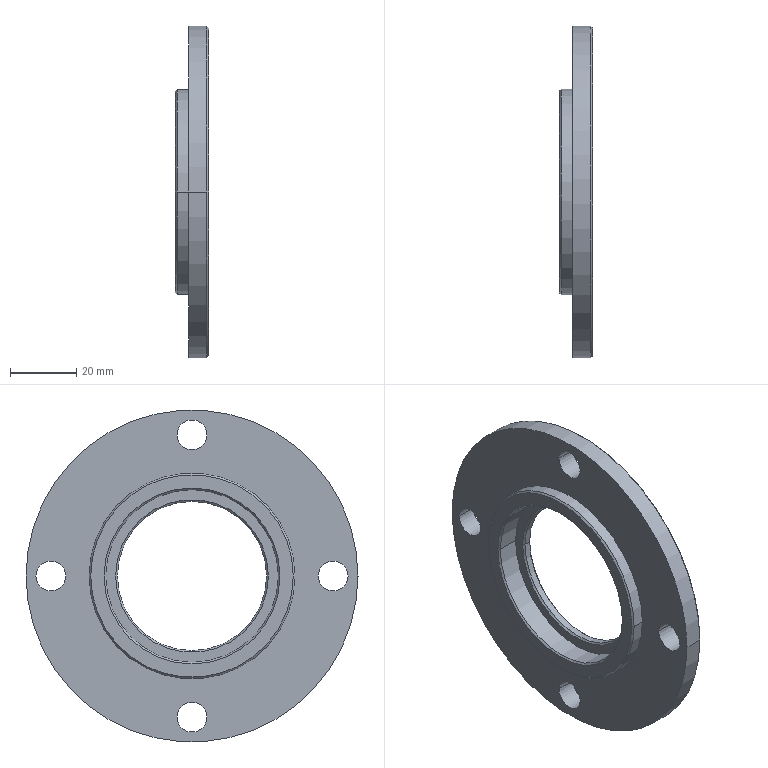Part | SolidWorks | features BaseBody 1 | 1 solid | 30 faces | box 10 x 100 x 100 mm | volume 37917 mm3 | cylinder 16 | cone 10 | plane 4 | commonest cylinder face diameters 9 x8 45 x2 52 x2 62 x2 100 x2
STEP:
#1=CARTESIAN_POINT('',(5.5,-22.5,0.));
#2=VERTEX_POINT('',#1);
#3=CARTESIAN_POINT('',(5.5,22.5,0.));
#4=VERTEX_POINT('',#3);
#5=CARTESIAN_POINT('',(5.5,0.,0.));
#6=DIRECTION('',(1.,0.,0.));
#7=DIRECTION('',(0.,-1.,0.));
#8=AXIS2_PLACEMENT_3D('',#5,#6,#7);
#9=CIRCLE('',#8,22.5);
#10=EDGE_CURVE('',#2,#4,#9,.T.);
#11=ORIENTED_EDGE('',*,*,#10,.F.);
#12=CARTESIAN_POINT('',(6.,-23.,0.));
#13=VERTEX_POINT('',#12);
#14=CARTESIAN_POINT('',(6.,-23.,0.));
#15=DIRECTION('',(0.7071,-0.7071,0.));
#16=VECTOR('',#15,1000.);
#17=LINE('',#14,#16);
#18=EDGE_CURVE('',#2,#13,#17,.T.);
#19=ORIENTED_EDGE('',*,*,#18,.T.);
#20=CARTESIAN_POINT('',(6.,23.,0.));
#21=VERTEX_POINT('',#20);
#22=CARTESIAN_POINT('',(6.,0.,0.));
#23=DIRECTION('',(-1.,0.,0.));
#24=DIRECTION('',(0.,1.,0.));
#25=AXIS2_PLACEMENT_3D('',#22,#23,#24);
#26=CIRCLE('',#25,23.);
#27=EDGE_CURVE('',#21,#13,#26,.T.);
#28=ORIENTED_EDGE('',*,*,#27,.F.);
#29=CARTESIAN_POINT('',(6.,23.,0.));
#30=DIRECTION('',(0.7071,0.7071,0.));
#31=VECTOR('',#30,1000.);
#32=LINE('',#29,#31);
#33=EDGE_CURVE('',#4,#21,#32,.T.);
#34=ORIENTED_EDGE('',*,*,#33,.F.);
#35=EDGE_LOOP('',(#11,#19,#28,#34));
#36=FACE_OUTER_BOUND('',#35,.T.);
#37=CARTESIAN_POINT('',(6.,0.,0.));
#38=DIRECTION('',(1.,0.,0.));
#39=DIRECTION('',(0.,1.,0.));
#40=AXIS2_PLACEMENT_3D('',#37,#38,#39);
#41=CONICAL_SURFACE('',#40,23.,0.7854);
#42=ADVANCED_FACE('',(#36),#41,.F.);
#43=CARTESIAN_POINT('',(6.,47.,0.));
#44=VERTEX_POINT('',#43);
#45=CARTESIAN_POINT('',(6.,38.,0.));
#46=VERTEX_POINT('',#45);
#47=CARTESIAN_POINT('',(6.,42.5,0.));
#48=DIRECTION('',(-1.,0.,0.));
#49=DIRECTION('',(0.,-1.,0.));
#50=AXIS2_PLACEMENT_3D('',#47,#48,#49);
#51=CIRCLE('',#50,4.5);
#52=EDGE_CURVE('',#44,#46,#51,.T.);
#53=ORIENTED_EDGE('',*,*,#52,.F.);
#54=CARTESIAN_POINT('',(0.,47.,0.));
#55=VERTEX_POINT('',#54);
#56=CARTESIAN_POINT('',(141.774,47.,0.));
#57=DIRECTION('',(-1.,0.,0.));
#58=VECTOR('',#57,1000.);
#59=LINE('',#56,#58);
#60=EDGE_CURVE('',#44,#55,#59,.T.);
#61=ORIENTED_EDGE('',*,*,#60,.T.);
#62=CARTESIAN_POINT('',(0.,38.,0.));
#63=VERTEX_POINT('',#62);
#64=CARTESIAN_POINT('',(0.,42.5,0.));
#65=DIRECTION('',(1.,0.,0.));
#66=DIRECTION('',(0.,-1.,0.));
#67=AXIS2_PLACEMENT_3D('',#64,#65,#66);
#68=CIRCLE('',#67,4.5);
#69=EDGE_CURVE('',#63,#55,#68,.T.);
#70=ORIENTED_EDGE('',*,*,#69,.F.);
#71=CARTESIAN_POINT('',(141.774,38.,0.));
#72=DIRECTION('',(-1.,0.,0.));
#73=VECTOR('',#72,1000.);
#74=LINE('',#71,#73);
#75=EDGE_CURVE('',#46,#63,#74,.T.);
#76=ORIENTED_EDGE('',*,*,#75,.F.);
#77=EDGE_LOOP('',(#53,#61,#70,#76));
#78=FACE_OUTER_BOUND('',#77,.T.);
#79=CARTESIAN_POINT('',(141.774,42.5,0.));
#80=DIRECTION('',(-1.,0.,0.));
#81=DIRECTION('',(0.,-1.,0.));
#82=AXIS2_PLACEMENT_3D('',#79,#80,#81);
#83=CYLINDRICAL_SURFACE('',#82,4.5);
#84=ADVANCED_FACE('',(#78),#83,.F.);
#85=CARTESIAN_POINT('',(6.,4.5,42.5));
#86=VERTEX_POINT('',#85);
#87=CARTESIAN_POINT('',(6.,-4.5,42.5));
#88=VERTEX_POINT('',#87);
#89=CARTESIAN_POINT('',(6.,0.,42.5));
#90=DIRECTION('',(-1.,0.,0.));
#91=DIRECTION('',(0.,-1.,0.));
#92=AXIS2_PLACEMENT_3D('',#89,#90,#91);
#93=CIRCLE('',#92,4.5);
#94=EDGE_CURVE('',#86,#88,#93,.T.);
#95=ORIENTED_EDGE('',*,*,#94,.F.);
#96=CARTESIAN_POINT('',(0.,4.5,42.5));
#97=VERTEX_POINT('',#96);
#98=CARTESIAN_POINT('',(141.774,4.5,42.5));
#99=DIRECTION('',(-1.,0.,0.));
#100=VECTOR('',#99,1000.);
#101=LINE('',#98,#100);
#102=EDGE_CURVE('',#86,#97,#101,.T.);
#103=ORIENTED_EDGE('',*,*,#102,.T.);
#104=CARTESIAN_POINT('',(0.,-4.5,42.5));
#105=VERTEX_POINT('',#104);
#106=CARTESIAN_POINT('',(0.,0.,42.5));
#107=DIRECTION('',(1.,0.,0.));
#108=DIRECTION('',(0.,-1.,0.));
#109=AXIS2_PLACEMENT_3D('',#106,#107,#108);
#110=CIRCLE('',#109,4.5);
#111=EDGE_CURVE('',#105,#97,#110,.T.);
#112=ORIENTED_EDGE('',*,*,#111,.F.);
#113=CARTESIAN_POINT('',(141.774,-4.5,42.5));
#114=DIRECTION('',(-1.,0.,0.));
#115=VECTOR('',#114,1000.);
#116=LINE('',#113,#115);
#117=EDGE_CURVE('',#88,#105,#116,.T.);
#118=ORIENTED_EDGE('',*,*,#117,.F.);
#119=EDGE_LOOP('',(#95,#103,#112,#118));
#120=FACE_OUTER_BOUND('',#119,.T.);
#121=CARTESIAN_POINT('',(141.774,0.,42.5));
#122=DIRECTION('',(-1.,0.,0.));
#123=DIRECTION('',(0.,-1.,0.));
#124=AXIS2_PLACEMENT_3D('',#121,#122,#123);
#125=CYLINDRICAL_SURFACE('',#124,4.5);
#126=ADVANCED_FACE('',(#120),#125,.F.);
#127=CARTESIAN_POINT('',(6.,-38.,0.));
#128=VERTEX_POINT('',#127);
#129=CARTESIAN_POINT('',(6.,-47.,0.));
#130=VERTEX_POINT('',#129);
#131=CARTESIAN_POINT('',(6.,-42.5,0.));
#132=DIRECTION('',(-1.,0.,0.));
#133=DIRECTION('',(0.,-1.,0.));
#134=AXIS2_PLACEMENT_3D('',#131,#132,#133);
#135=CIRCLE('',#134,4.5);
#136=EDGE_CURVE('',#128,#130,#135,.T.);
#137=ORIENTED_EDGE('',*,*,#136,.F.);
#138=CARTESIAN_POINT('',(0.,-38.,0.));
#139=VERTEX_POINT('',#138);
#140=CARTESIAN_POINT('',(141.774,-38.,0.));
#141=DIRECTION('',(-1.,0.,0.));
#142=VECTOR('',#141,1000.);
#143=LINE('',#140,#142);
#144=EDGE_CURVE('',#128,#139,#143,.T.);
#145=ORIENTED_EDGE('',*,*,#144,.T.);
#146=CARTESIAN_POINT('',(0.,-47.,0.));
#147=VERTEX_POINT('',#146);
#148=CARTESIAN_POINT('',(0.,-42.5,0.));
#149=DIRECTION('',(1.,0.,0.));
#150=DIRECTION('',(0.,-1.,0.));
#151=AXIS2_PLACEMENT_3D('',#148,#149,#150);
#152=CIRCLE('',#151,4.5);
#153=EDGE_CURVE('',#147,#139,#152,.T.);
#154=ORIENTED_EDGE('',*,*,#153,.F.);
#155=CARTESIAN_POINT('',(141.774,-47.,0.));
#156=DIRECTION('',(-1.,0.,0.));
#157=VECTOR('',#156,1000.);
#158=LINE('',#155,#157);
#159=EDGE_CURVE('',#130,#147,#158,.T.);
#160=ORIENTED_EDGE('',*,*,#159,.F.);
#161=EDGE_LOOP('',(#137,#145,#154,#160));
#162=FACE_OUTER_BOUND('',#161,.T.);
#163=CARTESIAN_POINT('',(141.774,-42.5,0.));
#164=DIRECTION('',(-1.,0.,0.));
#165=DIRECTION('',(0.,-1.,0.));
#166=AXIS2_PLACEMENT_3D('',#163,#164,#165);
#167=CYLINDRICAL_SURFACE('',#166,4.5);
#168=ADVANCED_FACE('',(#162),#167,.F.);
#169=CARTESIAN_POINT('',(6.,4.5,-42.5));
#170=VERTEX_POINT('',#169);
#171=CARTESIAN_POINT('',(6.,-4.5,-42.5));
#172=VERTEX_POINT('',#171);
#173=CARTESIAN_POINT('',(6.,0.,-42.5));
#174=DIRECTION('',(-1.,0.,0.));
#175=DIRECTION('',(0.,-1.,0.));
#176=AXIS2_PLACEMENT_3D('',#173,#174,#175);
#177=CIRCLE('',#176,4.5);
#178=EDGE_CURVE('',#170,#172,#177,.T.);
#179=ORIENTED_EDGE('',*,*,#178,.F.);
#180=CARTESIAN_POINT('',(0.,4.5,-42.5));
#181=VERTEX_POINT('',#180);
#182=CARTESIAN_POINT('',(141.774,4.5,-42.5));
#183=DIRECTION('',(-1.,0.,0.));
#184=VECTOR('',#183,1000.);
#185=LINE('',#182,#184);
#186=EDGE_CURVE('',#170,#181,#185,.T.);
#187=ORIENTED_EDGE('',*,*,#186,.T.);
#188=CARTESIAN_POINT('',(0.,-4.5,-42.5));
#189=VERTEX_POINT('',#188);
#190=CARTESIAN_POINT('',(0.,0.,-42.5));
#191=DIRECTION('',(1.,0.,0.));
#192=DIRECTION('',(0.,-1.,0.));
#193=AXIS2_PLACEMENT_3D('',#190,#191,#192);
#194=CIRCLE('',#193,4.5);
#195=EDGE_CURVE('',#189,#181,#194,.T.);
#196=ORIENTED_EDGE('',*,*,#195,.F.);
#197=CARTESIAN_POINT('',(141.774,-4.5,-42.5));
#198=DIRECTION('',(-1.,0.,0.));
#199=VECTOR('',#198,1000.);
#200=LINE('',#197,#199);
#201=EDGE_CURVE('',#172,#189,#200,.T.);
#202=ORIENTED_EDGE('',*,*,#201,.F.);
#203=EDGE_LOOP('',(#179,#187,#196,#202));
#204=FACE_OUTER_BOUND('',#203,.T.);
#205=CARTESIAN_POINT('',(141.774,0.,-42.5));
#206=DIRECTION('',(-1.,0.,0.));
#207=DIRECTION('',(0.,-1.,0.));
#208=AXIS2_PLACEMENT_3D('',#205,#206,#207);
#209=CYLINDRICAL_SURFACE('',#208,4.5);
#210=ADVANCED_FACE('',(#204),#209,.F.);
#211=CARTESIAN_POINT('',(6.,49.5,0.));
#212=VERTEX_POINT('',#211);
#213=CARTESIAN_POINT('',(6.,-49.5,0.));
#214=VERTEX_POINT('',#213);
#215=CARTESIAN_POINT('',(6.,0.,0.));
#216=DIRECTION('',(1.,0.,0.));
#217=DIRECTION('',(0.,-1.,0.));
#218=AXIS2_PLACEMENT_3D('',#215,#216,#217);
#219=CIRCLE('',#218,49.5);
#220=EDGE_CURVE('',#212,#214,#219,.T.);
#221=ORIENTED_EDGE('',*,*,#220,.F.);
#222=CARTESIAN_POINT('',(5.5,50.,0.));
#223=VERTEX_POINT('',#222);
#224=CARTESIAN_POINT('',(5.5,50.,0.));
#225=DIRECTION('',(-0.7071,0.7071,0.));
#226=VECTOR('',#225,1000.);
#227=LINE('',#224,#226);
#228=EDGE_CURVE('',#212,#223,#227,.T.);
#229=ORIENTED_EDGE('',*,*,#228,.T.);
#230=CARTESIAN_POINT('',(5.5,-50.,0.));
#231=VERTEX_POINT('',#230);
#232=CARTESIAN_POINT('',(5.5,0.,0.));
#233=DIRECTION('',(1.,0.,0.));
#234=DIRECTION('',(0.,-1.,0.));
#235=AXIS2_PLACEMENT_3D('',#232,#233,#234);
#236=CIRCLE('',#235,50.);
#237=EDGE_CURVE('',#223,#231,#236,.T.);
#238=ORIENTED_EDGE('',*,*,#237,.T.);
#239=CARTESIAN_POINT('',(5.5,-50.,0.));
#240=DIRECTION('',(-0.7071,-0.7071,0.));
#241=VECTOR('',#240,1000.);
#242=LINE('',#239,#241);
#243=EDGE_CURVE('',#214,#231,#242,.T.);
#244=ORIENTED_EDGE('',*,*,#243,.F.);
#245=EDGE_LOOP('',(#221,#229,#238,#244));
#246=FACE_OUTER_BOUND('',#245,.T.);
#247=CARTESIAN_POINT('',(5.5,0.,0.));
#248=DIRECTION('',(-1.,0.,0.));
#249=DIRECTION('',(0.,-1.,0.));
#250=AXIS2_PLACEMENT_3D('',#247,#248,#249);
#251=CONICAL_SURFACE('',#250,50.,0.7854);
#252=ADVANCED_FACE('',(#246),#251,.T.);
#253=CARTESIAN_POINT('',(3.5,-22.5,0.));
#254=VERTEX_POINT('',#253);
#255=CARTESIAN_POINT('',(3.5,22.5,0.));
#256=VERTEX_POINT('',#255);
#257=CARTESIAN_POINT('',(3.5,0.,0.));
#258=DIRECTION('',(1.,0.,0.));
#259=DIRECTION('',(0.,1.,0.));
#260=AXIS2_PLACEMENT_3D('',#257,#258,#259);
#261=CIRCLE('',#260,22.5);
#262=EDGE_CURVE('',#254,#256,#261,.T.);
#263=ORIENTED_EDGE('',*,*,#262,.F.);
#264=CARTESIAN_POINT('',(4.5,-22.5,0.));
#265=DIRECTION('',(1.,0.,0.));
#266=VECTOR('',#265,1000.);
#267=LINE('',#264,#266);
#268=EDGE_CURVE('',#254,#2,#267,.T.);
#269=ORIENTED_EDGE('',*,*,#268,.T.);
#270=ORIENTED_EDGE('',*,*,#10,.T.);
#271=CARTESIAN_POINT('',(4.5,22.5,0.));
#272=DIRECTION('',(1.,0.,0.));
#273=VECTOR('',#272,1000.);
#274=LINE('',#271,#273);
#275=EDGE_CURVE('',#256,#4,#274,.T.);
#276=ORIENTED_EDGE('',*,*,#275,.F.);
#277=EDGE_LOOP('',(#263,#269,#270,#276));
#278=FACE_OUTER_BOUND('',#277,.T.);
#279=CARTESIAN_POINT('',(4.5,0.,0.));
#280=DIRECTION('',(1.,0.,0.));
#281=DIRECTION('',(0.,1.,0.));
#282=AXIS2_PLACEMENT_3D('',#279,#280,#281);
#283=CYLINDRICAL_SURFACE('',#282,22.5);
#284=ADVANCED_FACE('',(#278),#283,.F.);
#285=CARTESIAN_POINT('',(0.,-50.,0.));
#286=VERTEX_POINT('',#285);
#287=CARTESIAN_POINT('',(0.,50.,0.));
#288=VERTEX_POINT('',#287);
#289=CARTESIAN_POINT('',(0.,0.,0.));
#290=DIRECTION('',(-1.,0.,0.));
#291=DIRECTION('',(0.,1.,0.));
#292=AXIS2_PLACEMENT_3D('',#289,#290,#291);
#293=CIRCLE('',#292,50.);
#294=EDGE_CURVE('',#286,#288,#293,.T.);
#295=ORIENTED_EDGE('',*,*,#294,.F.);
#296=CARTESIAN_POINT('',(3.,-50.,0.));
#297=DIRECTION('',(1.,0.,0.));
#298=VECTOR('',#297,1000.);
#299=LINE('',#296,#298);
#300=EDGE_CURVE('',#286,#231,#299,.T.);
#301=ORIENTED_EDGE('',*,*,#300,.T.);
#302=ORIENTED_EDGE('',*,*,#237,.F.);
#303=CARTESIAN_POINT('',(3.,50.,0.));
#304=DIRECTION('',(1.,0.,0.));
#305=VECTOR('',#304,1000.);
#306=LINE('',#303,#305);
#307=EDGE_CURVE('',#288,#223,#306,.T.);
#308=ORIENTED_EDGE('',*,*,#307,.F.);
#309=EDGE_LOOP('',(#295,#301,#302,#308));
#310=FACE_OUTER_BOUND('',#309,.T.);
#311=CARTESIAN_POINT('',(3.,0.,0.));
#312=DIRECTION('',(1.,0.,0.));
#313=DIRECTION('',(0.,1.,0.));
#314=AXIS2_PLACEMENT_3D('',#311,#312,#313);
#315=CYLINDRICAL_SURFACE('',#314,50.);
#316=ADVANCED_FACE('',(#310),#315,.T.);
#317=ORIENTED_EDGE('',*,*,#262,.T.);
#318=CARTESIAN_POINT('',(3.,23.,0.));
#319=VERTEX_POINT('',#318);
#320=CARTESIAN_POINT('',(3.,23.,0.));
#321=DIRECTION('',(-0.7071,0.7071,0.));
#322=VECTOR('',#321,1000.);
#323=LINE('',#320,#322);
#324=EDGE_CURVE('',#256,#319,#323,.T.);
#325=ORIENTED_EDGE('',*,*,#324,.T.);
#326=CARTESIAN_POINT('',(3.,-23.,0.));
#327=VERTEX_POINT('',#326);
#328=CARTESIAN_POINT('',(3.,0.,0.));
#329=DIRECTION('',(1.,0.,0.));
#330=DIRECTION('',(0.,-1.,0.));
#331=AXIS2_PLACEMENT_3D('',#328,#329,#330);
#332=CIRCLE('',#331,23.);
#333=EDGE_CURVE('',#327,#319,#332,.T.);
#334=ORIENTED_EDGE('',*,*,#333,.F.);
#335=CARTESIAN_POINT('',(3.,-23.,0.));
#336=DIRECTION('',(-0.7071,-0.7071,0.));
#337=VECTOR('',#336,1000.);
#338=LINE('',#335,#337);
#339=EDGE_CURVE('',#254,#327,#338,.T.);
#340=ORIENTED_EDGE('',*,*,#339,.F.);
#341=EDGE_LOOP('',(#317,#325,#334,#340));
#342=FACE_OUTER_BOUND('',#341,.T.);
#343=CARTESIAN_POINT('',(3.,0.,0.));
#344=DIRECTION('',(-1.,0.,0.));
#345=DIRECTION('',(0.,-1.,0.));
#346=AXIS2_PLACEMENT_3D('',#343,#344,#345);
#347=CONICAL_SURFACE('',#346,23.,0.7854);
#348=ADVANCED_FACE('',(#342),#347,.F.);
#349=CARTESIAN_POINT('',(-3.5,31.,0.));
#350=VERTEX_POINT('',#349);
#351=CARTESIAN_POINT('',(-3.5,-31.,0.));
#352=VERTEX_POINT('',#351);
#353=CARTESIAN_POINT('',(-3.5,0.,0.));
#354=DIRECTION('',(1.,0.,0.));
#355=DIRECTION('',(0.,1.,0.));
#356=AXIS2_PLACEMENT_3D('',#353,#354,#355);
#357=CIRCLE('',#356,31.);
#358=EDGE_CURVE('',#350,#352,#357,.T.);
#359=ORIENTED_EDGE('',*,*,#358,.T.);
#360=CARTESIAN_POINT('',(0.,-31.,0.));
#361=VERTEX_POINT('',#360);
#362=CARTESIAN_POINT('',(-2.,-31.,0.));
#363=DIRECTION('',(1.,0.,0.));
#364=VECTOR('',#363,1000.);
#365=LINE('',#362,#364);
#366=EDGE_CURVE('',#352,#361,#365,.T.);
#367=ORIENTED_EDGE('',*,*,#366,.T.);
#368=CARTESIAN_POINT('',(0.,31.,0.));
#369=VERTEX_POINT('',#368);
#370=CARTESIAN_POINT('',(0.,0.,0.));
#371=DIRECTION('',(1.,0.,0.));
#372=DIRECTION('',(0.,1.,0.));
#373=AXIS2_PLACEMENT_3D('',#370,#371,#372);
#374=CIRCLE('',#373,31.);
#375=EDGE_CURVE('',#369,#361,#374,.T.);
#376=ORIENTED_EDGE('',*,*,#375,.F.);
#377=CARTESIAN_POINT('',(-2.,31.,0.));
#378=DIRECTION('',(1.,0.,0.));
#379=VECTOR('',#378,1000.);
#380=LINE('',#377,#379);
#381=EDGE_CURVE('',#350,#369,#380,.T.);
#382=ORIENTED_EDGE('',*,*,#381,.F.);
#383=EDGE_LOOP('',(#359,#367,#376,#382));
#384=FACE_OUTER_BOUND('',#383,.T.);
#385=CARTESIAN_POINT('',(-2.,0.,0.));
#386=DIRECTION('',(1.,0.,0.));
#387=DIRECTION('',(0.,1.,0.));
#388=AXIS2_PLACEMENT_3D('',#385,#386,#387);
#389=CYLINDRICAL_SURFACE('',#388,31.);
#390=ADVANCED_FACE('',(#384),#389,.T.);
#391=CARTESIAN_POINT('',(-4.,30.5,0.));
#392=VERTEX_POINT('',#391);
#393=CARTESIAN_POINT('',(-4.,-30.5,0.));
#394=VERTEX_POINT('',#393);
#395=CARTESIAN_POINT('',(-4.,0.,0.));
#396=DIRECTION('',(1.,0.,0.));
#397=DIRECTION('',(0.,1.,0.));
#398=AXIS2_PLACEMENT_3D('',#395,#396,#397);
#399=CIRCLE('',#398,30.5);
#400=EDGE_CURVE('',#392,#394,#399,.T.);
#401=ORIENTED_EDGE('',*,*,#400,.T.);
#402=CARTESIAN_POINT('',(-3.5,-31.,0.));
#403=DIRECTION('',(0.7071,-0.7071,0.));
#404=VECTOR('',#403,1000.);
#405=LINE('',#402,#404);
#406=EDGE_CURVE('',#394,#352,#405,.T.);
#407=ORIENTED_EDGE('',*,*,#406,.T.);
#408=ORIENTED_EDGE('',*,*,#358,.F.);
#409=CARTESIAN_POINT('',(-3.5,31.,0.));
#410=DIRECTION('',(0.7071,0.7071,0.));
#411=VECTOR('',#410,1000.);
#412=LINE('',#409,#411);
#413=EDGE_CURVE('',#392,#350,#412,.T.);
#414=ORIENTED_EDGE('',*,*,#413,.F.);
#415=EDGE_LOOP('',(#401,#407,#408,#414));
#416=FACE_OUTER_BOUND('',#415,.T.);
#417=CARTESIAN_POINT('',(-3.5,0.,0.));
#418=DIRECTION('',(1.,0.,0.));
#419=DIRECTION('',(0.,1.,0.));
#420=AXIS2_PLACEMENT_3D('',#417,#418,#419);
#421=CONICAL_SURFACE('',#420,31.,0.7854);
#422=ADVANCED_FACE('',(#416),#421,.T.);
#423=CARTESIAN_POINT('',(-3.5,-26.,0.));
#424=VERTEX_POINT('',#423);
#425=CARTESIAN_POINT('',(-3.5,26.,0.));
#426=VERTEX_POINT('',#425);
#427=CARTESIAN_POINT('',(-3.5,0.,0.));
#428=DIRECTION('',(1.,0.,0.));
#429=DIRECTION('',(0.,1.,0.));
#430=AXIS2_PLACEMENT_3D('',#427,#428,#429);
#431=CIRCLE('',#430,26.);
#432=EDGE_CURVE('',#424,#426,#431,.T.);
#433=ORIENTED_EDGE('',*,*,#432,.F.);
#434=CARTESIAN_POINT('',(3.,-26.,0.));
#435=VERTEX_POINT('',#434);
#436=CARTESIAN_POINT('',(-0.5,-26.,0.));
#437=DIRECTION('',(1.,0.,0.));
#438=VECTOR('',#437,1000.);
#439=LINE('',#436,#438);
#440=EDGE_CURVE('',#424,#435,#439,.T.);
#441=ORIENTED_EDGE('',*,*,#440,.T.);
#442=CARTESIAN_POINT('',(3.,26.,0.));
#443=VERTEX_POINT('',#442);
#444=CARTESIAN_POINT('',(3.,0.,0.));
#445=DIRECTION('',(-1.,0.,0.));
#446=DIRECTION('',(0.,1.,0.));
#447=AXIS2_PLACEMENT_3D('',#444,#445,#446);
#448=CIRCLE('',#447,26.);
#449=EDGE_CURVE('',#443,#435,#448,.T.);
#450=ORIENTED_EDGE('',*,*,#449,.F.);
#451=CARTESIAN_POINT('',(-0.5,26.,0.));
#452=DIRECTION('',(1.,0.,0.));
#453=VECTOR('',#452,1000.);
#454=LINE('',#451,#453);
#455=EDGE_CURVE('',#426,#443,#454,.T.);
#456=ORIENTED_EDGE('',*,*,#455,.F.);
#457=EDGE_LOOP('',(#433,#441,#450,#456));
#458=FACE_OUTER_BOUND('',#457,.T.);
#459=CARTESIAN_POINT('',(-0.5,0.,0.));
#460=DIRECTION('',(1.,0.,0.));
#461=DIRECTION('',(0.,1.,0.));
#462=AXIS2_PLACEMENT_3D('',#459,#460,#461);
#463=CYLINDRICAL_SURFACE('',#462,26.);
#464=ADVANCED_FACE('',(#458),#463,.F.);
#465=ORIENTED_EDGE('',*,*,#432,.T.);
#466=CARTESIAN_POINT('',(-4.,26.5,0.));
#467=VERTEX_POINT('',#466);
#468=CARTESIAN_POINT('',(-4.,26.5,0.));
#469=DIRECTION('',(-0.7071,0.7071,0.));
#470=VECTOR('',#469,1000.);
#471=LINE('',#468,#470);
#472=EDGE_CURVE('',#426,#467,#471,.T.);
#473=ORIENTED_EDGE('',*,*,#472,.T.);
#474=CARTESIAN_POINT('',(-4.,-26.5,0.));
#475=VERTEX_POINT('',#474);
#476=CARTESIAN_POINT('',(-4.,0.,0.));
#477=DIRECTION('',(1.,0.,0.));
#478=DIRECTION('',(0.,-1.,0.));
#479=AXIS2_PLACEMENT_3D('',#476,#477,#478);
#480=CIRCLE('',#479,26.5);
#481=EDGE_CURVE('',#475,#467,#480,.T.);
#482=ORIENTED_EDGE('',*,*,#481,.F.);
#483=CARTESIAN_POINT('',(-4.,-26.5,0.));
#484=DIRECTION('',(-0.7071,-0.7071,0.));
#485=VECTOR('',#484,1000.);
#486=LINE('',#483,#485);
#487=EDGE_CURVE('',#424,#475,#486,.T.);
#488=ORIENTED_EDGE('',*,*,#487,.F.);
#489=EDGE_LOOP('',(#465,#473,#482,#488));
#490=FACE_OUTER_BOUND('',#489,.T.);
#491=CARTESIAN_POINT('',(-4.,0.,0.));
#492=DIRECTION('',(-1.,0.,0.));
#493=DIRECTION('',(0.,-1.,0.));
#494=AXIS2_PLACEMENT_3D('',#491,#492,#493);
#495=CONICAL_SURFACE('',#494,26.5,0.7854);
#496=ADVANCED_FACE('',(#490),#495,.F.);
#497=ORIENTED_EDGE('',*,*,#27,.T.);
#498=CARTESIAN_POINT('',(6.,0.,0.));
#499=DIRECTION('',(-1.,0.,0.));
#500=DIRECTION('',(0.,1.,0.));
#501=AXIS2_PLACEMENT_3D('',#498,#499,#500);
#502=CIRCLE('',#501,23.);
#503=EDGE_CURVE('',#13,#21,#502,.T.);
#504=ORIENTED_EDGE('',*,*,#503,.T.);
#505=EDGE_LOOP('',(#497,#504));
#506=FACE_BOUND('',#505,.T.);
#507=CARTESIAN_POINT('',(6.,42.5,0.));
#508=DIRECTION('',(-1.,0.,0.));
#509=DIRECTION('',(0.,-1.,0.));
#510=AXIS2_PLACEMENT_3D('',#507,#508,#509);
#511=CIRCLE('',#510,4.5);
#512=EDGE_CURVE('',#46,#44,#511,.T.);
#513=ORIENTED_EDGE('',*,*,#512,.T.);
#514=ORIENTED_EDGE('',*,*,#52,.T.);
#515=EDGE_LOOP('',(#513,#514));
#516=FACE_BOUND('',#515,.T.);
#517=CARTESIAN_POINT('',(6.,0.,42.5));
#518=DIRECTION('',(-1.,0.,0.));
#519=DIRECTION('',(0.,-1.,0.));
#520=AXIS2_PLACEMENT_3D('',#517,#518,#519);
#521=CIRCLE('',#520,4.5);
#522=EDGE_CURVE('',#88,#86,#521,.T.);
#523=ORIENTED_EDGE('',*,*,#522,.T.);
#524=ORIENTED_EDGE('',*,*,#94,.T.);
#525=EDGE_LOOP('',(#523,#524));
#526=FACE_BOUND('',#525,.T.);
#527=CARTESIAN_POINT('',(6.,-42.5,0.));
#528=DIRECTION('',(-1.,0.,0.));
#529=DIRECTION('',(0.,-1.,0.));
#530=AXIS2_PLACEMENT_3D('',#527,#528,#529);
#531=CIRCLE('',#530,4.5);
#532=EDGE_CURVE('',#130,#128,#531,.T.);
#533=ORIENTED_EDGE('',*,*,#532,.T.);
#534=ORIENTED_EDGE('',*,*,#136,.T.);
#535=EDGE_LOOP('',(#533,#534));
#536=FACE_BOUND('',#535,.T.);
#537=CARTESIAN_POINT('',(6.,0.,-42.5));
#538=DIRECTION('',(-1.,0.,0.));
#539=DIRECTION('',(0.,-1.,0.));
#540=AXIS2_PLACEMENT_3D('',#537,#538,#539);
#541=CIRCLE('',#540,4.5);
#542=EDGE_CURVE('',#172,#170,#541,.T.);
#543=ORIENTED_EDGE('',*,*,#542,.T.);
#544=ORIENTED_EDGE('',*,*,#178,.T.);
#545=EDGE_LOOP('',(#543,#544));
#546=FACE_BOUND('',#545,.T.);
#547=CARTESIAN_POINT('',(6.,0.,0.));
#548=DIRECTION('',(1.,0.,0.));
#549=DIRECTION('',(0.,-1.,0.));
#550=AXIS2_PLACEMENT_3D('',#547,#548,#549);
#551=CIRCLE('',#550,49.5);
#552=EDGE_CURVE('',#214,#212,#551,.T.);
#553=ORIENTED_EDGE('',*,*,#552,.T.);
#554=ORIENTED_EDGE('',*,*,#220,.T.);
#555=EDGE_LOOP('',(#553,#554));
#556=FACE_OUTER_BOUND('',#555,.T.);
#557=CARTESIAN_POINT('',(6.,22.5,0.));
#558=DIRECTION('',(1.,0.,0.));
#559=DIRECTION('',(0.,1.,0.));
#560=AXIS2_PLACEMENT_3D('',#557,#558,#559);
#561=PLANE('',#560);
#562=ADVANCED_FACE('',(#506,#516,#526,#536,#546,#556),#561,.T.);
#563=ORIENTED_EDGE('',*,*,#18,.F.);
#564=CARTESIAN_POINT('',(5.5,0.,0.));
#565=DIRECTION('',(1.,0.,0.));
#566=DIRECTION('',(0.,-1.,0.));
#567=AXIS2_PLACEMENT_3D('',#564,#565,#566);
#568=CIRCLE('',#567,22.5);
#569=EDGE_CURVE('',#4,#2,#568,.T.);
#570=ORIENTED_EDGE('',*,*,#569,.F.);
#571=ORIENTED_EDGE('',*,*,#33,.T.);
#572=ORIENTED_EDGE('',*,*,#503,.F.);
#573=EDGE_LOOP('',(#563,#570,#571,#572));
#574=FACE_OUTER_BOUND('',#573,.T.);
#575=CARTESIAN_POINT('',(6.,0.,0.));
#576=DIRECTION('',(1.,0.,0.));
#577=DIRECTION('',(0.,1.,0.));
#578=AXIS2_PLACEMENT_3D('',#575,#576,#577);
#579=CONICAL_SURFACE('',#578,23.,0.7854);
#580=ADVANCED_FACE('',(#574),#579,.F.);
#581=ORIENTED_EDGE('',*,*,#60,.F.);
#582=ORIENTED_EDGE('',*,*,#512,.F.);
#583=ORIENTED_EDGE('',*,*,#75,.T.);
#584=CARTESIAN_POINT('',(0.,42.5,0.));
#585=DIRECTION('',(1.,0.,0.));
#586=DIRECTION('',(0.,-1.,0.));
#587=AXIS2_PLACEMENT_3D('',#584,#585,#586);
#588=CIRCLE('',#587,4.5);
#589=EDGE_CURVE('',#55,#63,#588,.T.);
#590=ORIENTED_EDGE('',*,*,#589,.F.);
#591=EDGE_LOOP('',(#581,#582,#583,#590));
#592=FACE_OUTER_BOUND('',#591,.T.);
#593=CARTESIAN_POINT('',(141.774,42.5,0.));
#594=DIRECTION('',(-1.,0.,0.));
#595=DIRECTION('',(0.,-1.,0.));
#596=AXIS2_PLACEMENT_3D('',#593,#594,#595);
#597=CYLINDRICAL_SURFACE('',#596,4.5);
#598=ADVANCED_FACE('',(#592),#597,.F.);
#599=ORIENTED_EDGE('',*,*,#102,.F.);
#600=ORIENTED_EDGE('',*,*,#522,.F.);
#601=ORIENTED_EDGE('',*,*,#117,.T.);
#602=CARTESIAN_POINT('',(0.,0.,42.5));
#603=DIRECTION('',(1.,0.,0.));
#604=DIRECTION('',(0.,-1.,0.));
#605=AXIS2_PLACEMENT_3D('',#602,#603,#604);
#606=CIRCLE('',#605,4.5);
#607=EDGE_CURVE('',#97,#105,#606,.T.);
#608=ORIENTED_EDGE('',*,*,#607,.F.);
#609=EDGE_LOOP('',(#599,#600,#601,#608));
#610=FACE_OUTER_BOUND('',#609,.T.);
#611=CARTESIAN_POINT('',(141.774,0.,42.5));
#612=DIRECTION('',(-1.,0.,0.));
#613=DIRECTION('',(0.,-1.,0.));
#614=AXIS2_PLACEMENT_3D('',#611,#612,#613);
#615=CYLINDRICAL_SURFACE('',#614,4.5);
#616=ADVANCED_FACE('',(#610),#615,.F.);
#617=ORIENTED_EDGE('',*,*,#144,.F.);
#618=ORIENTED_EDGE('',*,*,#532,.F.);
#619=ORIENTED_EDGE('',*,*,#159,.T.);
#620=CARTESIAN_POINT('',(0.,-42.5,0.));
#621=DIRECTION('',(1.,0.,0.));
#622=DIRECTION('',(0.,-1.,0.));
#623=AXIS2_PLACEMENT_3D('',#620,#621,#622);
#624=CIRCLE('',#623,4.5);
#625=EDGE_CURVE('',#139,#147,#624,.T.);
#626=ORIENTED_EDGE('',*,*,#625,.F.);
#627=EDGE_LOOP('',(#617,#618,#619,#626));
#628=FACE_OUTER_BOUND('',#627,.T.);
#629=CARTESIAN_POINT('',(141.774,-42.5,0.));
#630=DIRECTION('',(-1.,0.,0.));
#631=DIRECTION('',(0.,-1.,0.));
#632=AXIS2_PLACEMENT_3D('',#629,#630,#631);
#633=CYLINDRICAL_SURFACE('',#632,4.5);
#634=ADVANCED_FACE('',(#628),#633,.F.);
#635=ORIENTED_EDGE('',*,*,#186,.F.);
#636=ORIENTED_EDGE('',*,*,#542,.F.);
#637=ORIENTED_EDGE('',*,*,#201,.T.);
#638=CARTESIAN_POINT('',(0.,0.,-42.5));
#639=DIRECTION('',(1.,0.,0.));
#640=DIRECTION('',(0.,-1.,0.));
#641=AXIS2_PLACEMENT_3D('',#638,#639,#640);
#642=CIRCLE('',#641,4.5);
#643=EDGE_CURVE('',#181,#189,#642,.T.);
#644=ORIENTED_EDGE('',*,*,#643,.F.);
#645=EDGE_LOOP('',(#635,#636,#637,#644));
#646=FACE_OUTER_BOUND('',#645,.T.);
#647=CARTESIAN_POINT('',(141.774,0.,-42.5));
#648=DIRECTION('',(-1.,0.,0.));
#649=DIRECTION('',(0.,-1.,0.));
#650=AXIS2_PLACEMENT_3D('',#647,#648,#649);
#651=CYLINDRICAL_SURFACE('',#650,4.5);
#652=ADVANCED_FACE('',(#646),#651,.F.);
#653=ORIENTED_EDGE('',*,*,#228,.F.);
#654=ORIENTED_EDGE('',*,*,#552,.F.);
#655=ORIENTED_EDGE('',*,*,#243,.T.);
#656=CARTESIAN_POINT('',(5.5,0.,0.));
#657=DIRECTION('',(1.,0.,0.));
#658=DIRECTION('',(0.,-1.,0.));
#659=AXIS2_PLACEMENT_3D('',#656,#657,#658);
#660=CIRCLE('',#659,50.);
#661=EDGE_CURVE('',#231,#223,#660,.T.);
#662=ORIENTED_EDGE('',*,*,#661,.T.);
#663=EDGE_LOOP('',(#653,#654,#655,#662));
#664=FACE_OUTER_BOUND('',#663,.T.);
#665=CARTESIAN_POINT('',(5.5,0.,0.));
#666=DIRECTION('',(-1.,0.,0.));
#667=DIRECTION('',(0.,-1.,0.));
#668=AXIS2_PLACEMENT_3D('',#665,#666,#667);
#669=CONICAL_SURFACE('',#668,50.,0.7854);
#670=ADVANCED_FACE('',(#664),#669,.T.);
#671=ORIENTED_EDGE('',*,*,#268,.F.);
#672=CARTESIAN_POINT('',(3.5,0.,0.));
#673=DIRECTION('',(1.,0.,0.));
#674=DIRECTION('',(0.,1.,0.));
#675=AXIS2_PLACEMENT_3D('',#672,#673,#674);
#676=CIRCLE('',#675,22.5);
#677=EDGE_CURVE('',#256,#254,#676,.T.);
#678=ORIENTED_EDGE('',*,*,#677,.F.);
#679=ORIENTED_EDGE('',*,*,#275,.T.);
#680=ORIENTED_EDGE('',*,*,#569,.T.);
#681=EDGE_LOOP('',(#671,#678,#679,#680));
#682=FACE_OUTER_BOUND('',#681,.T.);
#683=CARTESIAN_POINT('',(4.5,0.,0.));
#684=DIRECTION('',(1.,0.,0.));
#685=DIRECTION('',(0.,1.,0.));
#686=AXIS2_PLACEMENT_3D('',#683,#684,#685);
#687=CYLINDRICAL_SURFACE('',#686,22.5);
#688=ADVANCED_FACE('',(#682),#687,.F.);
#689=ORIENTED_EDGE('',*,*,#375,.T.);
#690=CARTESIAN_POINT('',(0.,0.,0.));
#691=DIRECTION('',(1.,0.,0.));
#692=DIRECTION('',(0.,1.,0.));
#693=AXIS2_PLACEMENT_3D('',#690,#691,#692);
#694=CIRCLE('',#693,31.);
#695=EDGE_CURVE('',#361,#369,#694,.T.);
#696=ORIENTED_EDGE('',*,*,#695,.T.);
#697=EDGE_LOOP('',(#689,#696));
#698=FACE_BOUND('',#697,.T.);
#699=ORIENTED_EDGE('',*,*,#69,.T.);
#700=ORIENTED_EDGE('',*,*,#589,.T.);
#701=EDGE_LOOP('',(#699,#700));
#702=FACE_BOUND('',#701,.T.);
#703=ORIENTED_EDGE('',*,*,#111,.T.);
#704=ORIENTED_EDGE('',*,*,#607,.T.);
#705=EDGE_LOOP('',(#703,#704));
#706=FACE_BOUND('',#705,.T.);
#707=ORIENTED_EDGE('',*,*,#153,.T.);
#708=ORIENTED_EDGE('',*,*,#625,.T.);
#709=EDGE_LOOP('',(#707,#708));
#710=FACE_BOUND('',#709,.T.);
#711=ORIENTED_EDGE('',*,*,#195,.T.);
#712=ORIENTED_EDGE('',*,*,#643,.T.);
#713=EDGE_LOOP('',(#711,#712));
#714=FACE_BOUND('',#713,.T.);
#715=CARTESIAN_POINT('',(0.,0.,0.));
#716=DIRECTION('',(-1.,0.,0.));
#717=DIRECTION('',(0.,1.,0.));
#718=AXIS2_PLACEMENT_3D('',#715,#716,#717);
#719=CIRCLE('',#718,50.);
#720=EDGE_CURVE('',#288,#286,#719,.T.);
#721=ORIENTED_EDGE('',*,*,#720,.T.);
#722=ORIENTED_EDGE('',*,*,#294,.T.);
#723=EDGE_LOOP('',(#721,#722));
#724=FACE_OUTER_BOUND('',#723,.T.);
#725=CARTESIAN_POINT('',(0.,50.,0.));
#726=DIRECTION('',(-1.,0.,0.));
#727=DIRECTION('',(0.,-1.,0.));
#728=AXIS2_PLACEMENT_3D('',#725,#726,#727);
#729=PLANE('',#728);
#730=ADVANCED_FACE('',(#698,#702,#706,#710,#714,#724),#729,.T.);
#731=ORIENTED_EDGE('',*,*,#300,.F.);
#732=ORIENTED_EDGE('',*,*,#720,.F.);
#733=ORIENTED_EDGE('',*,*,#307,.T.);
#734=ORIENTED_EDGE('',*,*,#661,.F.);
#735=EDGE_LOOP('',(#731,#732,#733,#734));
#736=FACE_OUTER_BOUND('',#735,.T.);
#737=CARTESIAN_POINT('',(3.,0.,0.));
#738=DIRECTION('',(1.,0.,0.));
#739=DIRECTION('',(0.,1.,0.));
#740=AXIS2_PLACEMENT_3D('',#737,#738,#739);
#741=CYLINDRICAL_SURFACE('',#740,50.);
#742=ADVANCED_FACE('',(#736),#741,.T.);
#743=ORIENTED_EDGE('',*,*,#324,.F.);
#744=ORIENTED_EDGE('',*,*,#677,.T.);
#745=ORIENTED_EDGE('',*,*,#339,.T.);
#746=CARTESIAN_POINT('',(3.,0.,0.));
#747=DIRECTION('',(1.,0.,0.));
#748=DIRECTION('',(0.,-1.,0.));
#749=AXIS2_PLACEMENT_3D('',#746,#747,#748);
#750=CIRCLE('',#749,23.);
#751=EDGE_CURVE('',#319,#327,#750,.T.);
#752=ORIENTED_EDGE('',*,*,#751,.F.);
#753=EDGE_LOOP('',(#743,#744,#745,#752));
#754=FACE_OUTER_BOUND('',#753,.T.);
#755=CARTESIAN_POINT('',(3.,0.,0.));
#756=DIRECTION('',(-1.,0.,0.));
#757=DIRECTION('',(0.,-1.,0.));
#758=AXIS2_PLACEMENT_3D('',#755,#756,#757);
#759=CONICAL_SURFACE('',#758,23.,0.7854);
#760=ADVANCED_FACE('',(#754),#759,.F.);
#761=ORIENTED_EDGE('',*,*,#366,.F.);
#762=CARTESIAN_POINT('',(-3.5,0.,0.));
#763=DIRECTION('',(1.,0.,0.));
#764=DIRECTION('',(0.,1.,0.));
#765=AXIS2_PLACEMENT_3D('',#762,#763,#764);
#766=CIRCLE('',#765,31.);
#767=EDGE_CURVE('',#352,#350,#766,.T.);
#768=ORIENTED_EDGE('',*,*,#767,.T.);
#769=ORIENTED_EDGE('',*,*,#381,.T.);
#770=ORIENTED_EDGE('',*,*,#695,.F.);
#771=EDGE_LOOP('',(#761,#768,#769,#770));
#772=FACE_OUTER_BOUND('',#771,.T.);
#773=CARTESIAN_POINT('',(-2.,0.,0.));
#774=DIRECTION('',(1.,0.,0.));
#775=DIRECTION('',(0.,1.,0.));
#776=AXIS2_PLACEMENT_3D('',#773,#774,#775);
#777=CYLINDRICAL_SURFACE('',#776,31.);
#778=ADVANCED_FACE('',(#772),#777,.T.);
#779=ORIENTED_EDGE('',*,*,#333,.T.);
#780=ORIENTED_EDGE('',*,*,#751,.T.);
#781=EDGE_LOOP('',(#779,#780));
#782=FACE_BOUND('',#781,.T.);
#783=ORIENTED_EDGE('',*,*,#449,.T.);
#784=CARTESIAN_POINT('',(3.,0.,0.));
#785=DIRECTION('',(-1.,0.,0.));
#786=DIRECTION('',(0.,1.,0.));
#787=AXIS2_PLACEMENT_3D('',#784,#785,#786);
#788=CIRCLE('',#787,26.);
#789=EDGE_CURVE('',#435,#443,#788,.T.);
#790=ORIENTED_EDGE('',*,*,#789,.T.);
#791=EDGE_LOOP('',(#783,#790));
#792=FACE_OUTER_BOUND('',#791,.T.);
#793=CARTESIAN_POINT('',(3.,26.,0.));
#794=DIRECTION('',(-1.,0.,0.));
#795=DIRECTION('',(0.,-1.,0.));
#796=AXIS2_PLACEMENT_3D('',#793,#794,#795);
#797=PLANE('',#796);
#798=ADVANCED_FACE('',(#782,#792),#797,.T.);
#799=ORIENTED_EDGE('',*,*,#406,.F.);
#800=CARTESIAN_POINT('',(-4.,0.,0.));
#801=DIRECTION('',(1.,0.,0.));
#802=DIRECTION('',(0.,1.,0.));
#803=AXIS2_PLACEMENT_3D('',#800,#801,#802);
#804=CIRCLE('',#803,30.5);
#805=EDGE_CURVE('',#394,#392,#804,.T.);
#806=ORIENTED_EDGE('',*,*,#805,.T.);
#807=ORIENTED_EDGE('',*,*,#413,.T.);
#808=ORIENTED_EDGE('',*,*,#767,.F.);
#809=EDGE_LOOP('',(#799,#806,#807,#808));
#810=FACE_OUTER_BOUND('',#809,.T.);
#811=CARTESIAN_POINT('',(-3.5,0.,0.));
#812=DIRECTION('',(1.,0.,0.));
#813=DIRECTION('',(0.,1.,0.));
#814=AXIS2_PLACEMENT_3D('',#811,#812,#813);
#815=CONICAL_SURFACE('',#814,31.,0.7854);
#816=ADVANCED_FACE('',(#810),#815,.T.);
#817=ORIENTED_EDGE('',*,*,#440,.F.);
#818=CARTESIAN_POINT('',(-3.5,0.,0.));
#819=DIRECTION('',(1.,0.,0.));
#820=DIRECTION('',(0.,1.,0.));
#821=AXIS2_PLACEMENT_3D('',#818,#819,#820);
#822=CIRCLE('',#821,26.);
#823=EDGE_CURVE('',#426,#424,#822,.T.);
#824=ORIENTED_EDGE('',*,*,#823,.F.);
#825=ORIENTED_EDGE('',*,*,#455,.T.);
#826=ORIENTED_EDGE('',*,*,#789,.F.);
#827=EDGE_LOOP('',(#817,#824,#825,#826));
#828=FACE_OUTER_BOUND('',#827,.T.);
#829=CARTESIAN_POINT('',(-0.5,0.,0.));
#830=DIRECTION('',(1.,0.,0.));
#831=DIRECTION('',(0.,1.,0.));
#832=AXIS2_PLACEMENT_3D('',#829,#830,#831);
#833=CYLINDRICAL_SURFACE('',#832,26.);
#834=ADVANCED_FACE('',(#828),#833,.F.);
#835=ORIENTED_EDGE('',*,*,#481,.T.);
#836=CARTESIAN_POINT('',(-4.,0.,0.));
#837=DIRECTION('',(1.,0.,0.));
#838=DIRECTION('',(0.,-1.,0.));
#839=AXIS2_PLACEMENT_3D('',#836,#837,#838);
#840=CIRCLE('',#839,26.5);
#841=EDGE_CURVE('',#467,#475,#840,.T.);
#842=ORIENTED_EDGE('',*,*,#841,.T.);
#843=EDGE_LOOP('',(#835,#842));
#844=FACE_BOUND('',#843,.T.);
#845=ORIENTED_EDGE('',*,*,#400,.F.);
#846=ORIENTED_EDGE('',*,*,#805,.F.);
#847=EDGE_LOOP('',(#845,#846));
#848=FACE_OUTER_BOUND('',#847,.T.);
#849=CARTESIAN_POINT('',(-4.,31.,0.));
#850=DIRECTION('',(-1.,0.,0.));
#851=DIRECTION('',(0.,-1.,0.));
#852=AXIS2_PLACEMENT_3D('',#849,#850,#851);
#853=PLANE('',#852);
#854=ADVANCED_FACE('',(#844,#848),#853,.T.);
#855=ORIENTED_EDGE('',*,*,#472,.F.);
#856=ORIENTED_EDGE('',*,*,#823,.T.);
#857=ORIENTED_EDGE('',*,*,#487,.T.);
#858=ORIENTED_EDGE('',*,*,#841,.F.);
#859=EDGE_LOOP('',(#855,#856,#857,#858));
#860=FACE_OUTER_BOUND('',#859,.T.);
#861=CARTESIAN_POINT('',(-4.,0.,0.));
#862=DIRECTION('',(-1.,0.,0.));
#863=DIRECTION('',(0.,-1.,0.));
#864=AXIS2_PLACEMENT_3D('',#861,#862,#863);
#865=CONICAL_SURFACE('',#864,26.5,0.7854);
#866=ADVANCED_FACE('',(#860),#865,.F.);
#867=CLOSED_SHELL('',(#42,#84,#126,#168,#210,#252,#284,#316,#348,#390,#422,#464,#496,#562,#580,#598,#616,#634,#652,#670,#688,#730,#742,#760,#778,#798,#816,#834,#854,#866));
#868=MANIFOLD_SOLID_BREP('',#867);
#869=CARTESIAN_POINT('',(0.,0.,0.));
#870=DIRECTION('',(0.,0.,1.));
#871=DIRECTION('',(1.,0.,0.));
#872=AXIS2_PLACEMENT_3D('',#869,#870,#871);
#873=(LENGTH_UNIT()NAMED_UNIT(*)SI_UNIT(.MILLI.,.METRE.));
#874=UNCERTAINTY_MEASURE_WITH_UNIT(LENGTH_MEASURE(0.00001),#873,'','');
#875=(NAMED_UNIT(*)PLANE_ANGLE_UNIT()SI_UNIT($,.RADIAN.));
#876=(NAMED_UNIT(*)SI_UNIT($,.STERADIAN.)SOLID_ANGLE_UNIT());
#877=(GEOMETRIC_REPRESENTATION_CONTEXT(3)GLOBAL_UNCERTAINTY_ASSIGNED_CONTEXT((#874))GLOBAL_UNIT_ASSIGNED_CONTEXT((#873,#875,#876))REPRESENTATION_CONTEXT('',''));
#878=ADVANCED_BREP_SHAPE_REPRESENTATION('',(#868,#872),#877);